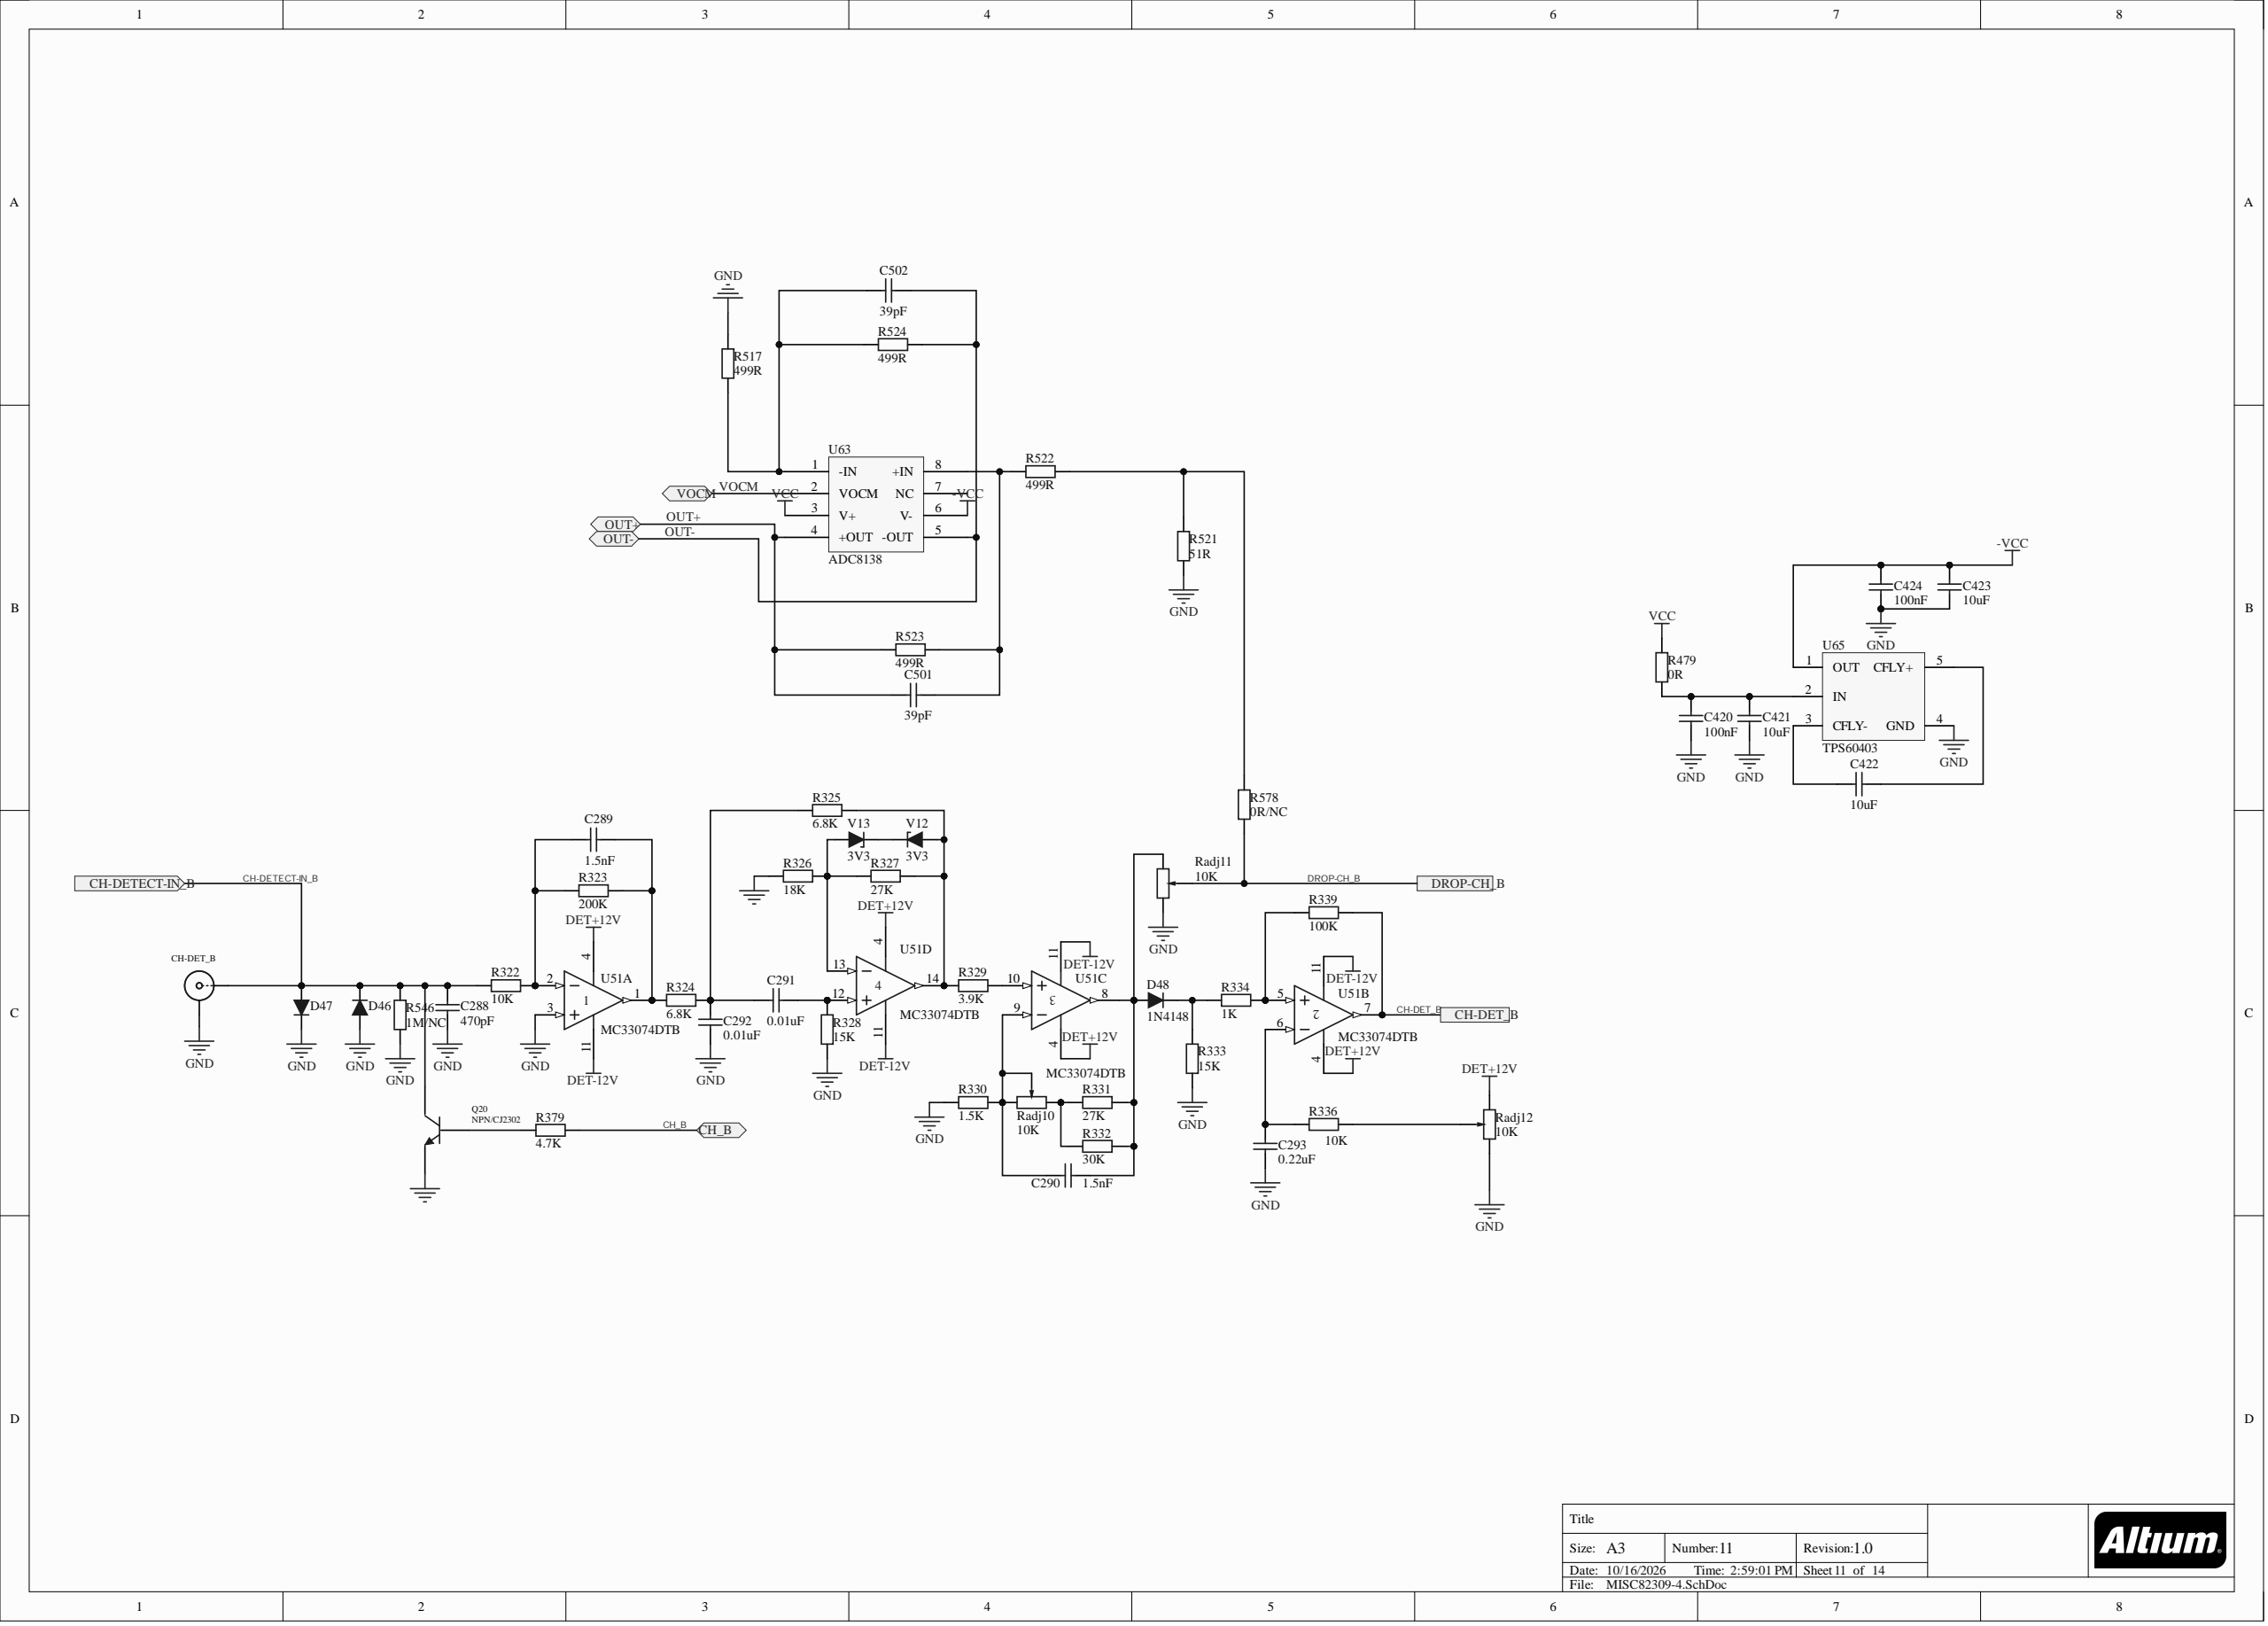Circuit board | Altium Designer | 747 parts | 576 nets | one sheet of the schematic
Parts on this sheet (reference | value | footprint):
C288 | 470pF | C0603
C289 | 1.5nF | C0603
C290 | 1.5nF | C0603
C291 | 0.01uF | C0603
C292 | 0.01uF | C0603
C293 | 0.22uF | C0603
C420 | 100nF | CAP_0603
C421 | 10uF | CAP_0603
C422 | 10uF | CAP_0603
C423 | 10uF | CAP_0603
C424 | 100nF | CAP_0603
C501 | 39pF | CAP_0603
C502 | 39pF | CAP_0603
CH-DET_B | SMB | SMB_V-RJ45
D46 | 1N4148WS | SOD323
D47 | 1N4148WS | SOD323
D48 | 1N4148 | SOD-323
Q20 | NPN/CJ2302 | SOT-23-3
R322 | 10K | RES_0603
R323 | 200K | RES_0603
R324 | 6.8K | RES_0603
R325 | 6.8K | RES_0603
R326 | 18K | RES_0603
R327 | 27K | RES_0603
R328 | 15K | RES_0603
R329 | 3.9K | RES_0603
R330 | 1.5K | RES_0603
R331 | 27K | RES_0603
R332 | 30K | RES_0603
R333 | 15K | RES_0603
R334 | 1K | RES_0603
R336 | 10K | RES_0603
R339 | 100K | RES_0603
R379 | 4.7K | RES_0603
R479 | 0R | RES_0603
R517 | 499R | RES_0603
R521 | 51R | RES_0603
R522 | 499R | RES_0603
R523 | 499R | RES_0603
R524 | 499R | RES_0603
R546 | 1M/NC | RES_0603
R578 | 0R/NC | RES_0603
Radj10 | 10K | Radj
Radj11 | 10K | Radj
Radj12 | 10K | Radj
U63 | ADC8138 | SO8_N
U65 | TPS60403 | SOT23-5_M
V12 | 3V3 | SOD-123
V13 | 3V3 | SOD-123
Nets of these parts (net: part-pin ...):
VOCM: U63-2
VCC: R479-2 U63-3
OUT-: C502-1 R524-1 U63-5
OUT+: C501-1 R523-1 U63-4
NetV12_2: V12-2 V13-2
NetR521_1: R521-1 R522-2 R578-2
NetR336_2: R336-2 Radj12-2
NetR334_2: R334-2 R339-1
NetR331_1: R331-1 R332-1 Radj10-1
NetR329_1: R329-1
NetR326_2: R326-2 R327-1 V13-1
NetR325_2: R325-2 R327-2 R329-2 V12-1
NetQ20_1: Q20-1 R379-1
NetD48_2: D48-2 R333-2 R334-1
NetC502_2: C502-2 R517-1 R524-2 U63-1
NetC501_2: C501-2 R522-1 R523-2 U63-8
NetC422_2: C422-2 U65-3
NetC422_1: C422-1 U65-5
NetC420_2: C420-2 C421-2 R479-1 U65-2
NetC293_1: C293-1 R336-1
NetC291_2: C291-2 C292-1 R324-2 R325-1
NetC291_1: C291-1 R328-2
NetC290_2: C290-2 R330-2 Radj10-2 Radj10-3
NetC290_1: C290-1 D48-1 R331-2 R332-2 Radj11-3
NetC289_2: C289-2 R322-2 R323-1
NetC289_1: C289-1 R323-2 R324-1
GND: C288-1 C292-2 C293-2 C420-1 C421-1 C423-2 C424-1 CH-DET_B-2 D46-1 D47-2 Q20-2 R326-1 R328-1 R330-1 R333-1 R517-2 R521-2 R546-1 Radj11-1 Radj12-1 U65-4
DROP-CH_B: R578-1 Radj11-2
DET+12V: Radj12-3
CH_B: R379-2
CH-DETECT-IN_B: C288-2 CH-DET_B-1 D46-2 D47-1 Q20-3 R322-1 R546-2
CH-DET_B: R339-2
-VCC: C423-1 C424-2 U63-6 U65-1